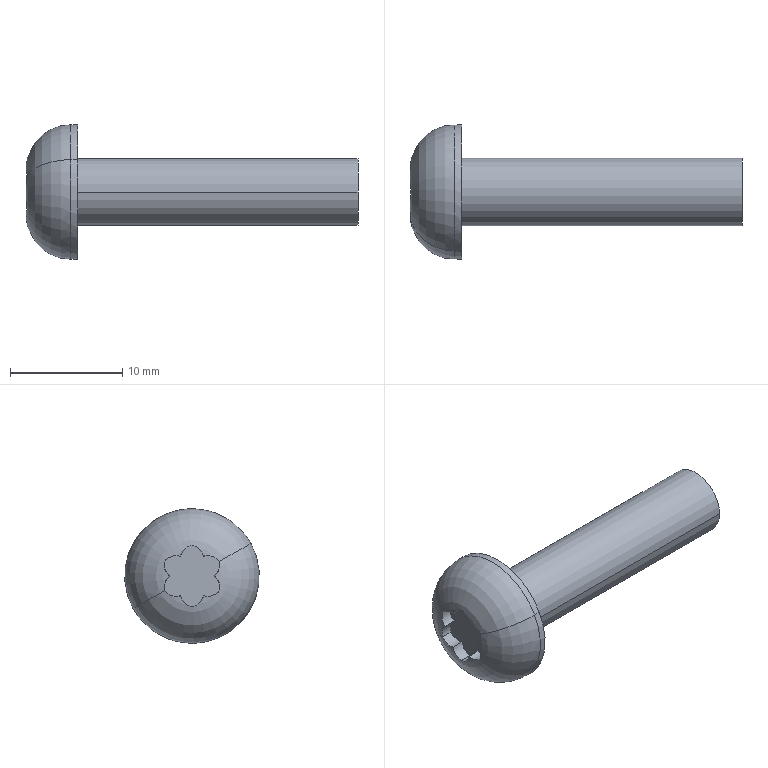Part | NX | features BREP 1 | 1 solid | 21 faces | box 29.6 x 12 x 12 mm | volume 1095 mm3 | cylinder 16 | plane 3 | torus 2 | commonest cylinder face diameters 2.56 x12 6 x2 12 x2
STEP:
#1=CARTESIAN_POINT('',(-3.48,0.,2.757));
#2=VERTEX_POINT('',#1);
#3=CARTESIAN_POINT('',(-3.48,1.012,1.754));
#4=VERTEX_POINT('',#3);
#5=CARTESIAN_POINT('',(-3.48,-0.2421,1.501));
#6=DIRECTION('',(-1.,0.,0.));
#7=DIRECTION('',(0.,0.,1.));
#8=AXIS2_PLACEMENT_3D('',#5,#6,#7);
#9=CIRCLE('',#8,1.28);
#10=EDGE_CURVE('',#2,#4,#9,.T.);
#11=ORIENTED_EDGE('',*,*,#10,.T.);
#12=CARTESIAN_POINT('',(-3.48,2.388,1.379));
#13=VERTEX_POINT('',#12);
#14=CARTESIAN_POINT('',(-3.48,1.421,0.5407));
#15=DIRECTION('',(-1.,0.,0.));
#16=DIRECTION('',(0.,0.,1.));
#17=AXIS2_PLACEMENT_3D('',#14,#15,#16);
#18=CIRCLE('',#17,1.28);
#19=EDGE_CURVE('',#4,#13,#18,.T.);
#20=ORIENTED_EDGE('',*,*,#19,.T.);
#21=CARTESIAN_POINT('',(-3.48,2.025,0.));
#22=VERTEX_POINT('',#21);
#23=CARTESIAN_POINT('',(-3.48,1.179,0.96));
#24=DIRECTION('',(-1.,0.,0.));
#25=DIRECTION('',(0.,0.,1.));
#26=AXIS2_PLACEMENT_3D('',#23,#24,#25);
#27=CIRCLE('',#26,1.28);
#28=EDGE_CURVE('',#13,#22,#27,.T.);
#29=ORIENTED_EDGE('',*,*,#28,.T.);
#30=CARTESIAN_POINT('',(-3.48,2.388,-1.379));
#31=VERTEX_POINT('',#30);
#32=CARTESIAN_POINT('',(-3.48,1.179,-0.96));
#33=DIRECTION('',(-1.,0.,0.));
#34=DIRECTION('',(0.,0.,1.));
#35=AXIS2_PLACEMENT_3D('',#32,#33,#34);
#36=CIRCLE('',#35,1.28);
#37=EDGE_CURVE('',#22,#31,#36,.T.);
#38=ORIENTED_EDGE('',*,*,#37,.T.);
#39=CARTESIAN_POINT('',(-3.48,1.012,-1.754));
#40=VERTEX_POINT('',#39);
#41=CARTESIAN_POINT('',(-3.48,1.421,-0.5407));
#42=DIRECTION('',(-1.,0.,0.));
#43=DIRECTION('',(0.,0.,1.));
#44=AXIS2_PLACEMENT_3D('',#41,#42,#43);
#45=CIRCLE('',#44,1.28);
#46=EDGE_CURVE('',#31,#40,#45,.T.);
#47=ORIENTED_EDGE('',*,*,#46,.T.);
#48=CARTESIAN_POINT('',(-3.48,0.,-2.757));
#49=VERTEX_POINT('',#48);
#50=CARTESIAN_POINT('',(-3.48,-0.2421,-1.501));
#51=DIRECTION('',(-1.,0.,0.));
#52=DIRECTION('',(0.,0.,1.));
#53=AXIS2_PLACEMENT_3D('',#50,#51,#52);
#54=CIRCLE('',#53,1.28);
#55=EDGE_CURVE('',#40,#49,#54,.T.);
#56=ORIENTED_EDGE('',*,*,#55,.T.);
#57=CARTESIAN_POINT('',(-3.48,-1.012,-1.754));
#58=VERTEX_POINT('',#57);
#59=CARTESIAN_POINT('',(-3.48,0.2421,-1.501));
#60=DIRECTION('',(-1.,0.,0.));
#61=DIRECTION('',(0.,0.,1.));
#62=AXIS2_PLACEMENT_3D('',#59,#60,#61);
#63=CIRCLE('',#62,1.28);
#64=EDGE_CURVE('',#49,#58,#63,.T.);
#65=ORIENTED_EDGE('',*,*,#64,.T.);
#66=CARTESIAN_POINT('',(-3.48,-2.388,-1.379));
#67=VERTEX_POINT('',#66);
#68=CARTESIAN_POINT('',(-3.48,-1.421,-0.5407));
#69=DIRECTION('',(-1.,0.,0.));
#70=DIRECTION('',(0.,0.,1.));
#71=AXIS2_PLACEMENT_3D('',#68,#69,#70);
#72=CIRCLE('',#71,1.28);
#73=EDGE_CURVE('',#58,#67,#72,.T.);
#74=ORIENTED_EDGE('',*,*,#73,.T.);
#75=CARTESIAN_POINT('',(-3.48,-2.025,0.));
#76=VERTEX_POINT('',#75);
#77=CARTESIAN_POINT('',(-3.48,-1.179,-0.96));
#78=DIRECTION('',(-1.,0.,0.));
#79=DIRECTION('',(0.,0.,1.));
#80=AXIS2_PLACEMENT_3D('',#77,#78,#79);
#81=CIRCLE('',#80,1.28);
#82=EDGE_CURVE('',#67,#76,#81,.T.);
#83=ORIENTED_EDGE('',*,*,#82,.T.);
#84=CARTESIAN_POINT('',(-3.48,-2.388,1.379));
#85=VERTEX_POINT('',#84);
#86=CARTESIAN_POINT('',(-3.48,-1.179,0.96));
#87=DIRECTION('',(-1.,0.,0.));
#88=DIRECTION('',(0.,0.,1.));
#89=AXIS2_PLACEMENT_3D('',#86,#87,#88);
#90=CIRCLE('',#89,1.28);
#91=EDGE_CURVE('',#76,#85,#90,.T.);
#92=ORIENTED_EDGE('',*,*,#91,.T.);
#93=CARTESIAN_POINT('',(-3.48,-1.012,1.754));
#94=VERTEX_POINT('',#93);
#95=CARTESIAN_POINT('',(-3.48,-1.421,0.5407));
#96=DIRECTION('',(-1.,0.,0.));
#97=DIRECTION('',(0.,0.,1.));
#98=AXIS2_PLACEMENT_3D('',#95,#96,#97);
#99=CIRCLE('',#98,1.28);
#100=EDGE_CURVE('',#85,#94,#99,.T.);
#101=ORIENTED_EDGE('',*,*,#100,.T.);
#102=CARTESIAN_POINT('',(-3.48,0.2421,1.501));
#103=DIRECTION('',(-1.,0.,0.));
#104=DIRECTION('',(0.,0.,1.));
#105=AXIS2_PLACEMENT_3D('',#102,#103,#104);
#106=CIRCLE('',#105,1.28);
#107=EDGE_CURVE('',#94,#2,#106,.T.);
#108=ORIENTED_EDGE('',*,*,#107,.T.);
#109=EDGE_LOOP('',(#11,#20,#29,#38,#47,#56,#65,#74,#83,#92,#101,#108));
#110=FACE_BOUND('',#109,.T.);
#111=CARTESIAN_POINT('',(-3.48,0.,0.));
#112=DIRECTION('',(-1.,0.,0.));
#113=DIRECTION('',(0.,-1.,0.));
#114=AXIS2_PLACEMENT_3D('',#111,#112,#113);
#115=PLANE('',#114);
#116=ADVANCED_FACE('',(#110),#115,.T.);
#117=CARTESIAN_POINT('',(-4.528,-0.000000134,2.758));
#118=VERTEX_POINT('',#117);
#119=CARTESIAN_POINT('',(-4.6,1.013,1.754));
#120=VERTEX_POINT('',#119);
#121=CARTESIAN_POINT('',(-4.528,0.,2.757));
#122=CARTESIAN_POINT('',(-4.53,0.06478,2.745));
#123=CARTESIAN_POINT('',(-4.538,0.2473,2.715));
#124=CARTESIAN_POINT('',(-4.584,0.8742,2.291));
#125=CARTESIAN_POINT('',(-4.599,0.9773,1.928));
#126=CARTESIAN_POINT('',(-4.6,1.012,1.754));
#127=B_SPLINE_CURVE_WITH_KNOTS('',3,(#121,#122,#123,#124,#125,#126),.UNSPECIFIED.,.F.,.F.,(4,1,1,4),(0.,0.25,0.5,1.),.UNSPECIFIED.);
#128=EDGE_CURVE('',#118,#120,#127,.T.);
#129=ORIENTED_EDGE('',*,*,#128,.T.);
#130=CARTESIAN_POINT('',(-4.04,1.012,1.754));
#131=DIRECTION('',(-1.,0.,0.));
#132=VECTOR('',#131,1000.);
#133=LINE('',#130,#132);
#134=EDGE_CURVE('',#4,#120,#133,.T.);
#135=ORIENTED_EDGE('',*,*,#134,.F.);
#136=ORIENTED_EDGE('',*,*,#10,.F.);
#137=CARTESIAN_POINT('',(-4.04,0.,2.757));
#138=DIRECTION('',(-1.,0.,0.));
#139=VECTOR('',#138,1000.);
#140=LINE('',#137,#139);
#141=EDGE_CURVE('',#2,#118,#140,.T.);
#142=ORIENTED_EDGE('',*,*,#141,.T.);
#143=EDGE_LOOP('',(#129,#135,#136,#142));
#144=FACE_BOUND('',#143,.T.);
#145=CARTESIAN_POINT('',(-4.04,-0.2421,1.501));
#146=DIRECTION('',(-1.,0.,0.));
#147=DIRECTION('',(0.,0.1892,0.9819));
#148=AXIS2_PLACEMENT_3D('',#145,#146,#147);
#149=CYLINDRICAL_SURFACE('',#148,1.28);
#150=ADVANCED_FACE('',(#144),#149,.F.);
#151=CARTESIAN_POINT('',(-4.528,2.388,1.379));
#152=VERTEX_POINT('',#151);
#153=CARTESIAN_POINT('',(-4.6,1.013,1.754));
#154=CARTESIAN_POINT('',(-4.599,1.181,1.811));
#155=CARTESIAN_POINT('',(-4.584,1.547,1.902));
#156=CARTESIAN_POINT('',(-4.538,2.227,1.572));
#157=CARTESIAN_POINT('',(-4.53,2.345,1.429));
#158=CARTESIAN_POINT('',(-4.528,2.388,1.379));
#159=B_SPLINE_CURVE_WITH_KNOTS('',3,(#153,#154,#155,#156,#157,#158),.UNSPECIFIED.,.F.,.F.,(4,1,1,4),(0.,0.5,0.75,1.),.UNSPECIFIED.);
#160=EDGE_CURVE('',#152,#120,#159,.F.);
#161=ORIENTED_EDGE('',*,*,#160,.F.);
#162=CARTESIAN_POINT('',(-4.04,2.388,1.379));
#163=DIRECTION('',(-1.,0.,0.));
#164=VECTOR('',#163,1000.);
#165=LINE('',#162,#164);
#166=EDGE_CURVE('',#13,#152,#165,.T.);
#167=ORIENTED_EDGE('',*,*,#166,.F.);
#168=ORIENTED_EDGE('',*,*,#19,.F.);
#169=ORIENTED_EDGE('',*,*,#134,.T.);
#170=EDGE_LOOP('',(#161,#167,#168,#169));
#171=FACE_BOUND('',#170,.T.);
#172=CARTESIAN_POINT('',(-4.04,1.421,0.5407));
#173=DIRECTION('',(-1.,0.,0.));
#174=DIRECTION('',(0.,-0.319,0.9478));
#175=AXIS2_PLACEMENT_3D('',#172,#173,#174);
#176=CYLINDRICAL_SURFACE('',#175,1.28);
#177=ADVANCED_FACE('',(#171),#176,.F.);
#178=CARTESIAN_POINT('',(-4.6,2.025,0.));
#179=VERTEX_POINT('',#178);
#180=CARTESIAN_POINT('',(-4.528,2.388,1.379));
#181=CARTESIAN_POINT('',(-4.53,2.41,1.316));
#182=CARTESIAN_POINT('',(-4.538,2.475,1.143));
#183=CARTESIAN_POINT('',(-4.584,2.421,0.3883));
#184=CARTESIAN_POINT('',(-4.599,2.159,0.1178));
#185=CARTESIAN_POINT('',(-4.6,2.025,0.));
#186=B_SPLINE_CURVE_WITH_KNOTS('',3,(#180,#181,#182,#183,#184,#185),.UNSPECIFIED.,.F.,.F.,(4,1,1,4),(0.000000175,0.25,0.5,1.),.UNSPECIFIED.);
#187=EDGE_CURVE('',#152,#179,#186,.T.);
#188=ORIENTED_EDGE('',*,*,#187,.T.);
#189=CARTESIAN_POINT('',(-4.04,2.025,0.));
#190=DIRECTION('',(-1.,0.,0.));
#191=VECTOR('',#190,1000.);
#192=LINE('',#189,#191);
#193=EDGE_CURVE('',#22,#179,#192,.T.);
#194=ORIENTED_EDGE('',*,*,#193,.F.);
#195=ORIENTED_EDGE('',*,*,#28,.F.);
#196=ORIENTED_EDGE('',*,*,#166,.T.);
#197=EDGE_LOOP('',(#188,#194,#195,#196));
#198=FACE_BOUND('',#197,.T.);
#199=CARTESIAN_POINT('',(-4.04,1.179,0.96));
#200=DIRECTION('',(-1.,0.,0.));
#201=DIRECTION('',(0.,0.945,0.3272));
#202=AXIS2_PLACEMENT_3D('',#199,#200,#201);
#203=CYLINDRICAL_SURFACE('',#202,1.28);
#204=ADVANCED_FACE('',(#198),#203,.F.);
#205=CARTESIAN_POINT('',(-4.53,2.408,-1.316));
#206=VERTEX_POINT('',#205);
#207=CARTESIAN_POINT('',(-4.6,2.025,0.));
#208=CARTESIAN_POINT('',(-4.599,2.156,-0.1159));
#209=CARTESIAN_POINT('',(-4.586,2.403,-0.3516));
#210=CARTESIAN_POINT('',(-4.54,2.478,-1.115));
#211=CARTESIAN_POINT('',(-4.532,2.422,-1.267));
#212=CARTESIAN_POINT('',(-4.53,2.408,-1.316));
#213=B_SPLINE_CURVE_WITH_KNOTS('',3,(#207,#208,#209,#210,#211,#212),.UNSPECIFIED.,.F.,.F.,(4,1,1,4),(0.,0.5,0.75,1.),.UNSPECIFIED.);
#214=EDGE_CURVE('',#206,#179,#213,.F.);
#215=ORIENTED_EDGE('',*,*,#214,.F.);
#216=CARTESIAN_POINT('',(-4.528,2.388,-1.379));
#217=VERTEX_POINT('',#216);
#218=CARTESIAN_POINT('',(-4.53,2.408,-1.316));
#219=CARTESIAN_POINT('',(-4.529,2.402,-1.337));
#220=CARTESIAN_POINT('',(-4.528,2.395,-1.358));
#221=CARTESIAN_POINT('',(-4.528,2.388,-1.379));
#222=B_SPLINE_CURVE_WITH_KNOTS('',3,(#218,#219,#220,#221),.UNSPECIFIED.,.F.,.F.,(4,4),(0.,1.),.UNSPECIFIED.);
#223=EDGE_CURVE('',#217,#206,#222,.F.);
#224=ORIENTED_EDGE('',*,*,#223,.F.);
#225=CARTESIAN_POINT('',(-4.04,2.388,-1.379));
#226=DIRECTION('',(-1.,0.,0.));
#227=VECTOR('',#226,1000.);
#228=LINE('',#225,#227);
#229=EDGE_CURVE('',#31,#217,#228,.T.);
#230=ORIENTED_EDGE('',*,*,#229,.F.);
#231=ORIENTED_EDGE('',*,*,#37,.F.);
#232=ORIENTED_EDGE('',*,*,#193,.T.);
#233=EDGE_LOOP('',(#215,#224,#230,#231,#232));
#234=FACE_BOUND('',#233,.T.);
#235=CARTESIAN_POINT('',(-4.04,1.179,-0.96));
#236=DIRECTION('',(-1.,0.,0.));
#237=DIRECTION('',(0.,0.6613,0.7501));
#238=AXIS2_PLACEMENT_3D('',#235,#236,#237);
#239=CYLINDRICAL_SURFACE('',#238,1.28);
#240=ADVANCED_FACE('',(#234),#239,.F.);
#241=CARTESIAN_POINT('',(-4.6,1.013,-1.754));
#242=VERTEX_POINT('',#241);
#243=CARTESIAN_POINT('',(-4.528,2.388,-1.379));
#244=CARTESIAN_POINT('',(-4.53,2.345,-1.429));
#245=CARTESIAN_POINT('',(-4.538,2.227,-1.572));
#246=CARTESIAN_POINT('',(-4.584,1.547,-1.902));
#247=CARTESIAN_POINT('',(-4.599,1.181,-1.811));
#248=CARTESIAN_POINT('',(-4.6,1.013,-1.754));
#249=B_SPLINE_CURVE_WITH_KNOTS('',3,(#243,#244,#245,#246,#247,#248),.UNSPECIFIED.,.F.,.F.,(4,1,1,4),(0.000000165,0.25,0.5,1.),.UNSPECIFIED.);
#250=EDGE_CURVE('',#217,#242,#249,.T.);
#251=ORIENTED_EDGE('',*,*,#250,.T.);
#252=CARTESIAN_POINT('',(-4.04,1.012,-1.754));
#253=DIRECTION('',(-1.,0.,0.));
#254=VECTOR('',#253,1000.);
#255=LINE('',#252,#254);
#256=EDGE_CURVE('',#40,#242,#255,.T.);
#257=ORIENTED_EDGE('',*,*,#256,.F.);
#258=ORIENTED_EDGE('',*,*,#46,.F.);
#259=ORIENTED_EDGE('',*,*,#229,.T.);
#260=EDGE_LOOP('',(#251,#257,#258,#259));
#261=FACE_BOUND('',#260,.T.);
#262=CARTESIAN_POINT('',(-4.04,1.421,-0.5407));
#263=DIRECTION('',(-1.,0.,0.));
#264=DIRECTION('',(0.,0.7558,-0.6548));
#265=AXIS2_PLACEMENT_3D('',#262,#263,#264);
#266=CYLINDRICAL_SURFACE('',#265,1.28);
#267=ADVANCED_FACE('',(#261),#266,.F.);
#268=CARTESIAN_POINT('',(-4.528,0.000000134,-2.758));
#269=VERTEX_POINT('',#268);
#270=CARTESIAN_POINT('',(-4.6,1.012,-1.754));
#271=CARTESIAN_POINT('',(-4.599,0.9773,-1.928));
#272=CARTESIAN_POINT('',(-4.584,0.8742,-2.291));
#273=CARTESIAN_POINT('',(-4.538,0.2473,-2.715));
#274=CARTESIAN_POINT('',(-4.53,0.06476,-2.745));
#275=CARTESIAN_POINT('',(-4.528,0.000000136,-2.757));
#276=B_SPLINE_CURVE_WITH_KNOTS('',3,(#270,#271,#272,#273,#274,#275),.UNSPECIFIED.,.F.,.F.,(4,1,1,4),(0.,0.5,0.75,1.),.UNSPECIFIED.);
#277=EDGE_CURVE('',#269,#242,#276,.F.);
#278=ORIENTED_EDGE('',*,*,#277,.F.);
#279=CARTESIAN_POINT('',(-4.04,0.,-2.757));
#280=DIRECTION('',(-1.,0.,0.));
#281=VECTOR('',#280,1000.);
#282=LINE('',#279,#281);
#283=EDGE_CURVE('',#49,#269,#282,.T.);
#284=ORIENTED_EDGE('',*,*,#283,.F.);
#285=ORIENTED_EDGE('',*,*,#55,.F.);
#286=ORIENTED_EDGE('',*,*,#256,.T.);
#287=EDGE_LOOP('',(#278,#284,#285,#286));
#288=FACE_BOUND('',#287,.T.);
#289=CARTESIAN_POINT('',(-4.04,-0.2421,-1.501));
#290=DIRECTION('',(-1.,0.,0.));
#291=DIRECTION('',(0.,0.9803,-0.1976));
#292=AXIS2_PLACEMENT_3D('',#289,#290,#291);
#293=CYLINDRICAL_SURFACE('',#292,1.28);
#294=ADVANCED_FACE('',(#288),#293,.F.);
#295=CARTESIAN_POINT('',(-4.6,-1.013,-1.754));
#296=VERTEX_POINT('',#295);
#297=CARTESIAN_POINT('',(-4.528,0.,-2.757));
#298=CARTESIAN_POINT('',(-4.53,-0.06478,-2.745));
#299=CARTESIAN_POINT('',(-4.538,-0.2473,-2.715));
#300=CARTESIAN_POINT('',(-4.584,-0.8742,-2.291));
#301=CARTESIAN_POINT('',(-4.599,-0.9773,-1.928));
#302=CARTESIAN_POINT('',(-4.6,-1.012,-1.754));
#303=B_SPLINE_CURVE_WITH_KNOTS('',3,(#297,#298,#299,#300,#301,#302),.UNSPECIFIED.,.F.,.F.,(4,1,1,4),(0.,0.25,0.5,1.),.UNSPECIFIED.);
#304=EDGE_CURVE('',#269,#296,#303,.T.);
#305=ORIENTED_EDGE('',*,*,#304,.T.);
#306=CARTESIAN_POINT('',(-4.04,-1.012,-1.754));
#307=DIRECTION('',(-1.,0.,0.));
#308=VECTOR('',#307,1000.);
#309=LINE('',#306,#308);
#310=EDGE_CURVE('',#58,#296,#309,.T.);
#311=ORIENTED_EDGE('',*,*,#310,.F.);
#312=ORIENTED_EDGE('',*,*,#64,.F.);
#313=ORIENTED_EDGE('',*,*,#283,.T.);
#314=EDGE_LOOP('',(#305,#311,#312,#313));
#315=FACE_BOUND('',#314,.T.);
#316=CARTESIAN_POINT('',(-4.04,0.2421,-1.501));
#317=DIRECTION('',(-1.,0.,0.));
#318=DIRECTION('',(0.,-0.1892,-0.9819));
#319=AXIS2_PLACEMENT_3D('',#316,#317,#318);
#320=CYLINDRICAL_SURFACE('',#319,1.28);
#321=ADVANCED_FACE('',(#315),#320,.F.);
#322=CARTESIAN_POINT('',(-4.528,-2.388,-1.379));
#323=VERTEX_POINT('',#322);
#324=CARTESIAN_POINT('',(-4.6,-1.013,-1.754));
#325=CARTESIAN_POINT('',(-4.599,-1.181,-1.811));
#326=CARTESIAN_POINT('',(-4.584,-1.547,-1.902));
#327=CARTESIAN_POINT('',(-4.538,-2.227,-1.572));
#328=CARTESIAN_POINT('',(-4.53,-2.345,-1.429));
#329=CARTESIAN_POINT('',(-4.528,-2.388,-1.379));
#330=B_SPLINE_CURVE_WITH_KNOTS('',3,(#324,#325,#326,#327,#328,#329),.UNSPECIFIED.,.F.,.F.,(4,1,1,4),(0.,0.5,0.75,1.),.UNSPECIFIED.);
#331=EDGE_CURVE('',#323,#296,#330,.F.);
#332=ORIENTED_EDGE('',*,*,#331,.F.);
#333=CARTESIAN_POINT('',(-4.04,-2.388,-1.379));
#334=DIRECTION('',(-1.,0.,0.));
#335=VECTOR('',#334,1000.);
#336=LINE('',#333,#335);
#337=EDGE_CURVE('',#67,#323,#336,.T.);
#338=ORIENTED_EDGE('',*,*,#337,.F.);
#339=ORIENTED_EDGE('',*,*,#73,.F.);
#340=ORIENTED_EDGE('',*,*,#310,.T.);
#341=EDGE_LOOP('',(#332,#338,#339,#340));
#342=FACE_BOUND('',#341,.T.);
#343=CARTESIAN_POINT('',(-4.04,-1.421,-0.5407));
#344=DIRECTION('',(-1.,0.,0.));
#345=DIRECTION('',(0.,0.319,-0.9478));
#346=AXIS2_PLACEMENT_3D('',#343,#344,#345);
#347=CYLINDRICAL_SURFACE('',#346,1.28);
#348=ADVANCED_FACE('',(#342),#347,.F.);
#349=CARTESIAN_POINT('',(-4.6,-2.025,0.));
#350=VERTEX_POINT('',#349);
#351=CARTESIAN_POINT('',(-4.528,-2.388,-1.379));
#352=CARTESIAN_POINT('',(-4.53,-2.41,-1.316));
#353=CARTESIAN_POINT('',(-4.538,-2.475,-1.143));
#354=CARTESIAN_POINT('',(-4.584,-2.421,-0.3883));
#355=CARTESIAN_POINT('',(-4.599,-2.159,-0.1178));
#356=CARTESIAN_POINT('',(-4.6,-2.025,0.));
#357=B_SPLINE_CURVE_WITH_KNOTS('',3,(#351,#352,#353,#354,#355,#356),.UNSPECIFIED.,.F.,.F.,(4,1,1,4),(0.000000175,0.25,0.5,1.),.UNSPECIFIED.);
#358=EDGE_CURVE('',#323,#350,#357,.T.);
#359=ORIENTED_EDGE('',*,*,#358,.T.);
#360=CARTESIAN_POINT('',(-4.04,-2.025,0.));
#361=DIRECTION('',(-1.,0.,0.));
#362=VECTOR('',#361,1000.);
#363=LINE('',#360,#362);
#364=EDGE_CURVE('',#76,#350,#363,.T.);
#365=ORIENTED_EDGE('',*,*,#364,.F.);
#366=ORIENTED_EDGE('',*,*,#82,.F.);
#367=ORIENTED_EDGE('',*,*,#337,.T.);
#368=EDGE_LOOP('',(#359,#365,#366,#367));
#369=FACE_BOUND('',#368,.T.);
#370=CARTESIAN_POINT('',(-4.04,-1.179,-0.96));
#371=DIRECTION('',(-1.,0.,0.));
#372=DIRECTION('',(0.,-0.945,-0.3272));
#373=AXIS2_PLACEMENT_3D('',#370,#371,#372);
#374=CYLINDRICAL_SURFACE('',#373,1.28);
#375=ADVANCED_FACE('',(#369),#374,.F.);
#376=CARTESIAN_POINT('',(-4.53,-2.408,1.316));
#377=VERTEX_POINT('',#376);
#378=CARTESIAN_POINT('',(-4.6,-2.025,0.));
#379=CARTESIAN_POINT('',(-4.599,-2.156,0.1159));
#380=CARTESIAN_POINT('',(-4.586,-2.403,0.3516));
#381=CARTESIAN_POINT('',(-4.54,-2.478,1.115));
#382=CARTESIAN_POINT('',(-4.532,-2.422,1.267));
#383=CARTESIAN_POINT('',(-4.53,-2.408,1.316));
#384=B_SPLINE_CURVE_WITH_KNOTS('',3,(#378,#379,#380,#381,#382,#383),.UNSPECIFIED.,.F.,.F.,(4,1,1,4),(0.,0.5,0.75,1.),.UNSPECIFIED.);
#385=EDGE_CURVE('',#377,#350,#384,.F.);
#386=ORIENTED_EDGE('',*,*,#385,.F.);
#387=CARTESIAN_POINT('',(-4.528,-2.388,1.379));
#388=VERTEX_POINT('',#387);
#389=CARTESIAN_POINT('',(-4.53,-2.408,1.316));
#390=CARTESIAN_POINT('',(-4.529,-2.402,1.337));
#391=CARTESIAN_POINT('',(-4.528,-2.395,1.358));
#392=CARTESIAN_POINT('',(-4.528,-2.388,1.379));
#393=B_SPLINE_CURVE_WITH_KNOTS('',3,(#389,#390,#391,#392),.UNSPECIFIED.,.F.,.F.,(4,4),(0.,1.),.UNSPECIFIED.);
#394=EDGE_CURVE('',#388,#377,#393,.F.);
#395=ORIENTED_EDGE('',*,*,#394,.F.);
#396=CARTESIAN_POINT('',(-4.04,-2.388,1.379));
#397=DIRECTION('',(-1.,0.,0.));
#398=VECTOR('',#397,1000.);
#399=LINE('',#396,#398);
#400=EDGE_CURVE('',#85,#388,#399,.T.);
#401=ORIENTED_EDGE('',*,*,#400,.F.);
#402=ORIENTED_EDGE('',*,*,#91,.F.);
#403=ORIENTED_EDGE('',*,*,#364,.T.);
#404=EDGE_LOOP('',(#386,#395,#401,#402,#403));
#405=FACE_BOUND('',#404,.T.);
#406=CARTESIAN_POINT('',(-4.04,-1.179,0.96));
#407=DIRECTION('',(-1.,0.,0.));
#408=DIRECTION('',(0.,-0.6613,-0.7501));
#409=AXIS2_PLACEMENT_3D('',#406,#407,#408);
#410=CYLINDRICAL_SURFACE('',#409,1.28);
#411=ADVANCED_FACE('',(#405),#410,.F.);
#412=CARTESIAN_POINT('',(-4.6,-1.013,1.754));
#413=VERTEX_POINT('',#412);
#414=CARTESIAN_POINT('',(-4.528,-2.388,1.379));
#415=CARTESIAN_POINT('',(-4.53,-2.345,1.429));
#416=CARTESIAN_POINT('',(-4.538,-2.227,1.572));
#417=CARTESIAN_POINT('',(-4.584,-1.547,1.902));
#418=CARTESIAN_POINT('',(-4.599,-1.181,1.811));
#419=CARTESIAN_POINT('',(-4.6,-1.013,1.754));
#420=B_SPLINE_CURVE_WITH_KNOTS('',3,(#414,#415,#416,#417,#418,#419),.UNSPECIFIED.,.F.,.F.,(4,1,1,4),(0.000000165,0.25,0.5,1.),.UNSPECIFIED.);
#421=EDGE_CURVE('',#388,#413,#420,.T.);
#422=ORIENTED_EDGE('',*,*,#421,.T.);
#423=CARTESIAN_POINT('',(-4.04,-1.012,1.754));
#424=DIRECTION('',(-1.,0.,0.));
#425=VECTOR('',#424,1000.);
#426=LINE('',#423,#425);
#427=EDGE_CURVE('',#94,#413,#426,.T.);
#428=ORIENTED_EDGE('',*,*,#427,.F.);
#429=ORIENTED_EDGE('',*,*,#100,.F.);
#430=ORIENTED_EDGE('',*,*,#400,.T.);
#431=EDGE_LOOP('',(#422,#428,#429,#430));
#432=FACE_BOUND('',#431,.T.);
#433=CARTESIAN_POINT('',(-4.04,-1.421,0.5407));
#434=DIRECTION('',(-1.,0.,0.));
#435=DIRECTION('',(0.,-0.7558,0.6548));
#436=AXIS2_PLACEMENT_3D('',#433,#434,#435);
#437=CYLINDRICAL_SURFACE('',#436,1.28);
#438=ADVANCED_FACE('',(#432),#437,.F.);
#439=CARTESIAN_POINT('',(-4.6,-1.012,1.754));
#440=CARTESIAN_POINT('',(-4.599,-0.9773,1.928));
#441=CARTESIAN_POINT('',(-4.584,-0.8742,2.291));
#442=CARTESIAN_POINT('',(-4.538,-0.2473,2.715));
#443=CARTESIAN_POINT('',(-4.53,-0.06476,2.745));
#444=CARTESIAN_POINT('',(-4.528,-0.000000136,2.757));
#445=B_SPLINE_CURVE_WITH_KNOTS('',3,(#439,#440,#441,#442,#443,#444),.UNSPECIFIED.,.F.,.F.,(4,1,1,4),(0.,0.5,0.75,1.),.UNSPECIFIED.);
#446=EDGE_CURVE('',#118,#413,#445,.F.);
#447=ORIENTED_EDGE('',*,*,#446,.F.);
#448=ORIENTED_EDGE('',*,*,#141,.F.);
#449=ORIENTED_EDGE('',*,*,#107,.F.);
#450=ORIENTED_EDGE('',*,*,#427,.T.);
#451=EDGE_LOOP('',(#447,#448,#449,#450));
#452=FACE_BOUND('',#451,.T.);
#453=CARTESIAN_POINT('',(-4.04,0.2421,1.501));
#454=DIRECTION('',(-1.,0.,0.));
#455=DIRECTION('',(0.,-0.9803,0.1976));
#456=AXIS2_PLACEMENT_3D('',#453,#454,#455);
#457=CYLINDRICAL_SURFACE('',#456,1.28);
#458=ADVANCED_FACE('',(#452),#457,.F.);
#459=CARTESIAN_POINT('',(-0.6,-5.265,2.877));
#460=VERTEX_POINT('',#459);
#461=CARTESIAN_POINT('',(-0.6,5.265,-2.877));
#462=VERTEX_POINT('',#461);
#463=CARTESIAN_POINT('',(-0.6,5.265,-2.877));
#464=CARTESIAN_POINT('',(-0.6,6.019,-1.498));
#465=CARTESIAN_POINT('',(-0.6,6.379,1.87));
#466=CARTESIAN_POINT('',(-0.6,3.188,5.836));
#467=CARTESIAN_POINT('',(-0.6,-1.873,6.379));
#468=CARTESIAN_POINT('',(-0.6,-4.512,4.255));
#469=CARTESIAN_POINT('',(-0.6,-5.265,2.877));
#470=B_SPLINE_CURVE_WITH_KNOTS('',3,(#463,#464,#465,#466,#467,#468,#469),.UNSPECIFIED.,.F.,.F.,(4,1,1,1,4),(0.,0.25,0.5,0.75,1.),.UNSPECIFIED.);
#471=EDGE_CURVE('',#460,#462,#470,.F.);
#472=ORIENTED_EDGE('',*,*,#471,.F.);
#473=CARTESIAN_POINT('',(0.,-5.265,2.877));
#474=VERTEX_POINT('',#473);
#475=CARTESIAN_POINT('',(-0.3,-5.265,2.877));
#476=DIRECTION('',(-1.,0.,0.));
#477=VECTOR('',#476,1000.);
#478=LINE('',#475,#477);
#479=EDGE_CURVE('',#474,#460,#478,.T.);
#480=ORIENTED_EDGE('',*,*,#479,.F.);
#481=CARTESIAN_POINT('',(0.,5.265,-2.877));
#482=VERTEX_POINT('',#481);
#483=CARTESIAN_POINT('',(0.,0.,0.));
#484=DIRECTION('',(-1.,0.,0.));
#485=DIRECTION('',(0.,0.,1.));
#486=AXIS2_PLACEMENT_3D('',#483,#484,#485);
#487=CIRCLE('',#486,6.);
#488=EDGE_CURVE('',#474,#482,#487,.T.);
#489=ORIENTED_EDGE('',*,*,#488,.T.);
#490=CARTESIAN_POINT('',(-0.3,5.265,-2.877));
#491=DIRECTION('',(-1.,0.,0.));
#492=VECTOR('',#491,1000.);
#493=LINE('',#490,#492);
#494=EDGE_CURVE('',#482,#462,#493,.T.);
#495=ORIENTED_EDGE('',*,*,#494,.T.);
#496=EDGE_LOOP('',(#472,#480,#489,#495));
#497=FACE_BOUND('',#496,.T.);
#498=CARTESIAN_POINT('',(-2.3,0.,0.));
#499=DIRECTION('',(-1.,0.,0.));
#500=DIRECTION('',(0.,-0.8776,0.4794));
#501=AXIS2_PLACEMENT_3D('',#498,#499,#500);
#502=CYLINDRICAL_SURFACE('',#501,6.);
#503=ADVANCED_FACE('',(#497),#502,.T.);
#504=CARTESIAN_POINT('',(-0.6,-5.265,2.877));
#505=CARTESIAN_POINT('',(-0.6,-6.019,1.498));
#506=CARTESIAN_POINT('',(-0.6,-6.379,-1.87));
#507=CARTESIAN_POINT('',(-0.6,-3.188,-5.836));
#508=CARTESIAN_POINT('',(-0.6,1.873,-6.379));
#509=CARTESIAN_POINT('',(-0.6,4.512,-4.255));
#510=CARTESIAN_POINT('',(-0.6,5.265,-2.877));
#511=B_SPLINE_CURVE_WITH_KNOTS('',3,(#504,#505,#506,#507,#508,#509,#510),.UNSPECIFIED.,.F.,.F.,(4,1,1,1,4),(0.,0.25,0.5,0.75,1.),.UNSPECIFIED.);
#512=EDGE_CURVE('',#462,#460,#511,.F.);
#513=ORIENTED_EDGE('',*,*,#512,.F.);
#514=ORIENTED_EDGE('',*,*,#494,.F.);
#515=CARTESIAN_POINT('',(0.,0.,0.));
#516=DIRECTION('',(-1.,0.,0.));
#517=DIRECTION('',(0.,0.,1.));
#518=AXIS2_PLACEMENT_3D('',#515,#516,#517);
#519=CIRCLE('',#518,6.);
#520=EDGE_CURVE('',#482,#474,#519,.T.);
#521=ORIENTED_EDGE('',*,*,#520,.T.);
#522=ORIENTED_EDGE('',*,*,#479,.T.);
#523=EDGE_LOOP('',(#513,#514,#521,#522));
#524=FACE_BOUND('',#523,.T.);
#525=CARTESIAN_POINT('',(-2.3,0.,0.));
#526=DIRECTION('',(-1.,0.,0.));
#527=DIRECTION('',(0.,-0.8776,0.4794));
#528=AXIS2_PLACEMENT_3D('',#525,#526,#527);
#529=CYLINDRICAL_SURFACE('',#528,6.);
#530=ADVANCED_FACE('',(#524),#529,.T.);
#531=CARTESIAN_POINT('',(-4.53,-2.408,1.316));
#532=CARTESIAN_POINT('',(-4.359,-3.204,1.75));
#533=CARTESIAN_POINT('',(-3.363,-4.682,2.558));
#534=CARTESIAN_POINT('',(-1.522,-5.266,2.877));
#535=CARTESIAN_POINT('',(-0.6,-5.266,2.877));
#536=B_SPLINE_CURVE_WITH_KNOTS('',3,(#531,#532,#533,#534,#535),.UNSPECIFIED.,.F.,.F.,(4,1,4),(0.,0.5,1.),.UNSPECIFIED.);
#537=EDGE_CURVE('',#460,#377,#536,.F.);
#538=ORIENTED_EDGE('',*,*,#537,.F.);
#539=ORIENTED_EDGE('',*,*,#471,.T.);
#540=CARTESIAN_POINT('',(-0.6,5.266,-2.877));
#541=CARTESIAN_POINT('',(-1.522,5.266,-2.877));
#542=CARTESIAN_POINT('',(-3.363,4.682,-2.558));
#543=CARTESIAN_POINT('',(-4.359,3.204,-1.75));
#544=CARTESIAN_POINT('',(-4.53,2.408,-1.316));
#545=B_SPLINE_CURVE_WITH_KNOTS('',3,(#540,#541,#542,#543,#544),.UNSPECIFIED.,.F.,.F.,(4,1,4),(0.,0.5,1.),.UNSPECIFIED.);
#546=EDGE_CURVE('',#462,#206,#545,.T.);
#547=ORIENTED_EDGE('',*,*,#546,.T.);
#548=ORIENTED_EDGE('',*,*,#214,.T.);
#549=ORIENTED_EDGE('',*,*,#187,.F.);
#550=ORIENTED_EDGE('',*,*,#160,.T.);
#551=ORIENTED_EDGE('',*,*,#128,.F.);
#552=ORIENTED_EDGE('',*,*,#446,.T.);
#553=ORIENTED_EDGE('',*,*,#421,.F.);
#554=ORIENTED_EDGE('',*,*,#394,.T.);
#555=EDGE_LOOP('',(#538,#539,#547,#548,#549,#550,#551,#552,#553,#554));
#556=FACE_BOUND('',#555,.T.);
#557=CARTESIAN_POINT('',(-0.5998,0.,0.));
#558=DIRECTION('',(1.,0.,0.));
#559=DIRECTION('',(0.,0.,-1.));
#560=AXIS2_PLACEMENT_3D('',#557,#558,#559);
#561=DEGENERATE_TOROIDAL_SURFACE('',#560,2.,4.,.T.);
#562=ADVANCED_FACE('',(#556),#561,.T.);
#563=ORIENTED_EDGE('',*,*,#546,.F.);
#564=ORIENTED_EDGE('',*,*,#512,.T.);
#565=ORIENTED_EDGE('',*,*,#537,.T.);
#566=ORIENTED_EDGE('',*,*,#385,.T.);
#567=ORIENTED_EDGE('',*,*,#358,.F.);
#568=ORIENTED_EDGE('',*,*,#331,.T.);
#569=ORIENTED_EDGE('',*,*,#304,.F.);
#570=ORIENTED_EDGE('',*,*,#277,.T.);
#571=ORIENTED_EDGE('',*,*,#250,.F.);
#572=ORIENTED_EDGE('',*,*,#223,.T.);
#573=EDGE_LOOP('',(#563,#564,#565,#566,#567,#568,#569,#570,#571,#572));
#574=FACE_BOUND('',#573,.T.);
#575=CARTESIAN_POINT('',(-0.5998,0.,0.));
#576=DIRECTION('',(1.,0.,0.));
#577=DIRECTION('',(0.,0.,-1.));
#578=AXIS2_PLACEMENT_3D('',#575,#576,#577);
#579=DEGENERATE_TOROIDAL_SURFACE('',#578,2.,4.,.T.);
#580=ADVANCED_FACE('',(#574),#579,.T.);
#581=CARTESIAN_POINT('',(0.,-3.,0.));
#582=VERTEX_POINT('',#581);
#583=CARTESIAN_POINT('',(0.,3.,0.));
#584=VERTEX_POINT('',#583);
#585=CARTESIAN_POINT('',(0.,0.,0.));
#586=DIRECTION('',(1.,0.,0.));
#587=DIRECTION('',(0.,0.,-1.));
#588=AXIS2_PLACEMENT_3D('',#585,#586,#587);
#589=CIRCLE('',#588,3.);
#590=EDGE_CURVE('',#582,#584,#589,.T.);
#591=ORIENTED_EDGE('',*,*,#590,.F.);
#592=CARTESIAN_POINT('',(0.,0.,0.));
#593=DIRECTION('',(1.,0.,0.));
#594=DIRECTION('',(0.,0.,-1.));
#595=AXIS2_PLACEMENT_3D('',#592,#593,#594);
#596=CIRCLE('',#595,3.);
#597=EDGE_CURVE('',#584,#582,#596,.T.);
#598=ORIENTED_EDGE('',*,*,#597,.F.);
#599=EDGE_LOOP('',(#591,#598));
#600=FACE_BOUND('',#599,.T.);
#601=ORIENTED_EDGE('',*,*,#488,.F.);
#602=ORIENTED_EDGE('',*,*,#520,.F.);
#603=EDGE_LOOP('',(#601,#602));
#604=FACE_BOUND('',#603,.T.);
#605=CARTESIAN_POINT('',(0.,0.,0.));
#606=DIRECTION('',(-1.,0.,0.));
#607=DIRECTION('',(0.,1.,0.));
#608=AXIS2_PLACEMENT_3D('',#605,#606,#607);
#609=PLANE('',#608);
#610=ADVANCED_FACE('',(#600,#604),#609,.F.);
#611=CARTESIAN_POINT('',(25.,3.,0.));
#612=VERTEX_POINT('',#611);
#613=CARTESIAN_POINT('',(25.,-3.,0.));
#614=VERTEX_POINT('',#613);
#615=CARTESIAN_POINT('',(25.,0.,0.));
#616=DIRECTION('',(1.,0.,0.));
#617=DIRECTION('',(0.,0.,-1.));
#618=AXIS2_PLACEMENT_3D('',#615,#616,#617);
#619=CIRCLE('',#618,3.);
#620=EDGE_CURVE('',#612,#614,#619,.T.);
#621=ORIENTED_EDGE('',*,*,#620,.T.);
#622=CARTESIAN_POINT('',(25.,0.,0.));
#623=DIRECTION('',(1.,0.,0.));
#624=DIRECTION('',(0.,0.,-1.));
#625=AXIS2_PLACEMENT_3D('',#622,#623,#624);
#626=CIRCLE('',#625,3.);
#627=EDGE_CURVE('',#614,#612,#626,.T.);
#628=ORIENTED_EDGE('',*,*,#627,.T.);
#629=EDGE_LOOP('',(#621,#628));
#630=FACE_BOUND('',#629,.T.);
#631=CARTESIAN_POINT('',(25.,0.,0.));
#632=DIRECTION('',(1.,0.,0.));
#633=DIRECTION('',(0.,1.,0.));
#634=AXIS2_PLACEMENT_3D('',#631,#632,#633);
#635=PLANE('',#634);
#636=ADVANCED_FACE('',(#630),#635,.T.);
#637=CARTESIAN_POINT('',(12.5,-3.,0.));
#638=DIRECTION('',(1.,0.,0.));
#639=VECTOR('',#638,1000.);
#640=LINE('',#637,#639);
#641=EDGE_CURVE('',#582,#614,#640,.T.);
#642=ORIENTED_EDGE('',*,*,#641,.F.);
#643=ORIENTED_EDGE('',*,*,#590,.T.);
#644=CARTESIAN_POINT('',(12.5,3.,0.));
#645=DIRECTION('',(1.,0.,0.));
#646=VECTOR('',#645,1000.);
#647=LINE('',#644,#646);
#648=EDGE_CURVE('',#584,#612,#647,.T.);
#649=ORIENTED_EDGE('',*,*,#648,.T.);
#650=ORIENTED_EDGE('',*,*,#627,.F.);
#651=EDGE_LOOP('',(#642,#643,#649,#650));
#652=FACE_BOUND('',#651,.T.);
#653=CARTESIAN_POINT('',(12.5,0.,0.));
#654=DIRECTION('',(1.,0.,0.));
#655=DIRECTION('',(0.,1.,0.));
#656=AXIS2_PLACEMENT_3D('',#653,#654,#655);
#657=CYLINDRICAL_SURFACE('',#656,3.);
#658=ADVANCED_FACE('',(#652),#657,.T.);
#659=ORIENTED_EDGE('',*,*,#648,.F.);
#660=ORIENTED_EDGE('',*,*,#597,.T.);
#661=ORIENTED_EDGE('',*,*,#641,.T.);
#662=ORIENTED_EDGE('',*,*,#620,.F.);
#663=EDGE_LOOP('',(#659,#660,#661,#662));
#664=FACE_BOUND('',#663,.T.);
#665=CARTESIAN_POINT('',(12.5,0.,0.));
#666=DIRECTION('',(1.,0.,0.));
#667=DIRECTION('',(0.,1.,0.));
#668=AXIS2_PLACEMENT_3D('',#665,#666,#667);
#669=CYLINDRICAL_SURFACE('',#668,3.);
#670=ADVANCED_FACE('',(#664),#669,.T.);
#671=CLOSED_SHELL('',(#116,#150,#177,#204,#240,#267,#294,#321,#348,#375,#411,#438,#458,#503,#530,#562,#580,#610,#636,#658,#670));
#672=MANIFOLD_SOLID_BREP('',#671);
#673=(LENGTH_UNIT()NAMED_UNIT(*)SI_UNIT(.MILLI.,.METRE.));
#674=UNCERTAINTY_MEASURE_WITH_UNIT(LENGTH_MEASURE(0.0508),#673,'','');
#675=(NAMED_UNIT(*)PLANE_ANGLE_UNIT()SI_UNIT($,.RADIAN.));
#676=(NAMED_UNIT(*)SI_UNIT($,.STERADIAN.)SOLID_ANGLE_UNIT());
#677=(GEOMETRIC_REPRESENTATION_CONTEXT(3)GLOBAL_UNCERTAINTY_ASSIGNED_CONTEXT((#674))GLOBAL_UNIT_ASSIGNED_CONTEXT((#673,#675,#676))REPRESENTATION_CONTEXT('',''));
#678=ADVANCED_BREP_SHAPE_REPRESENTATION('',(#672),#677);